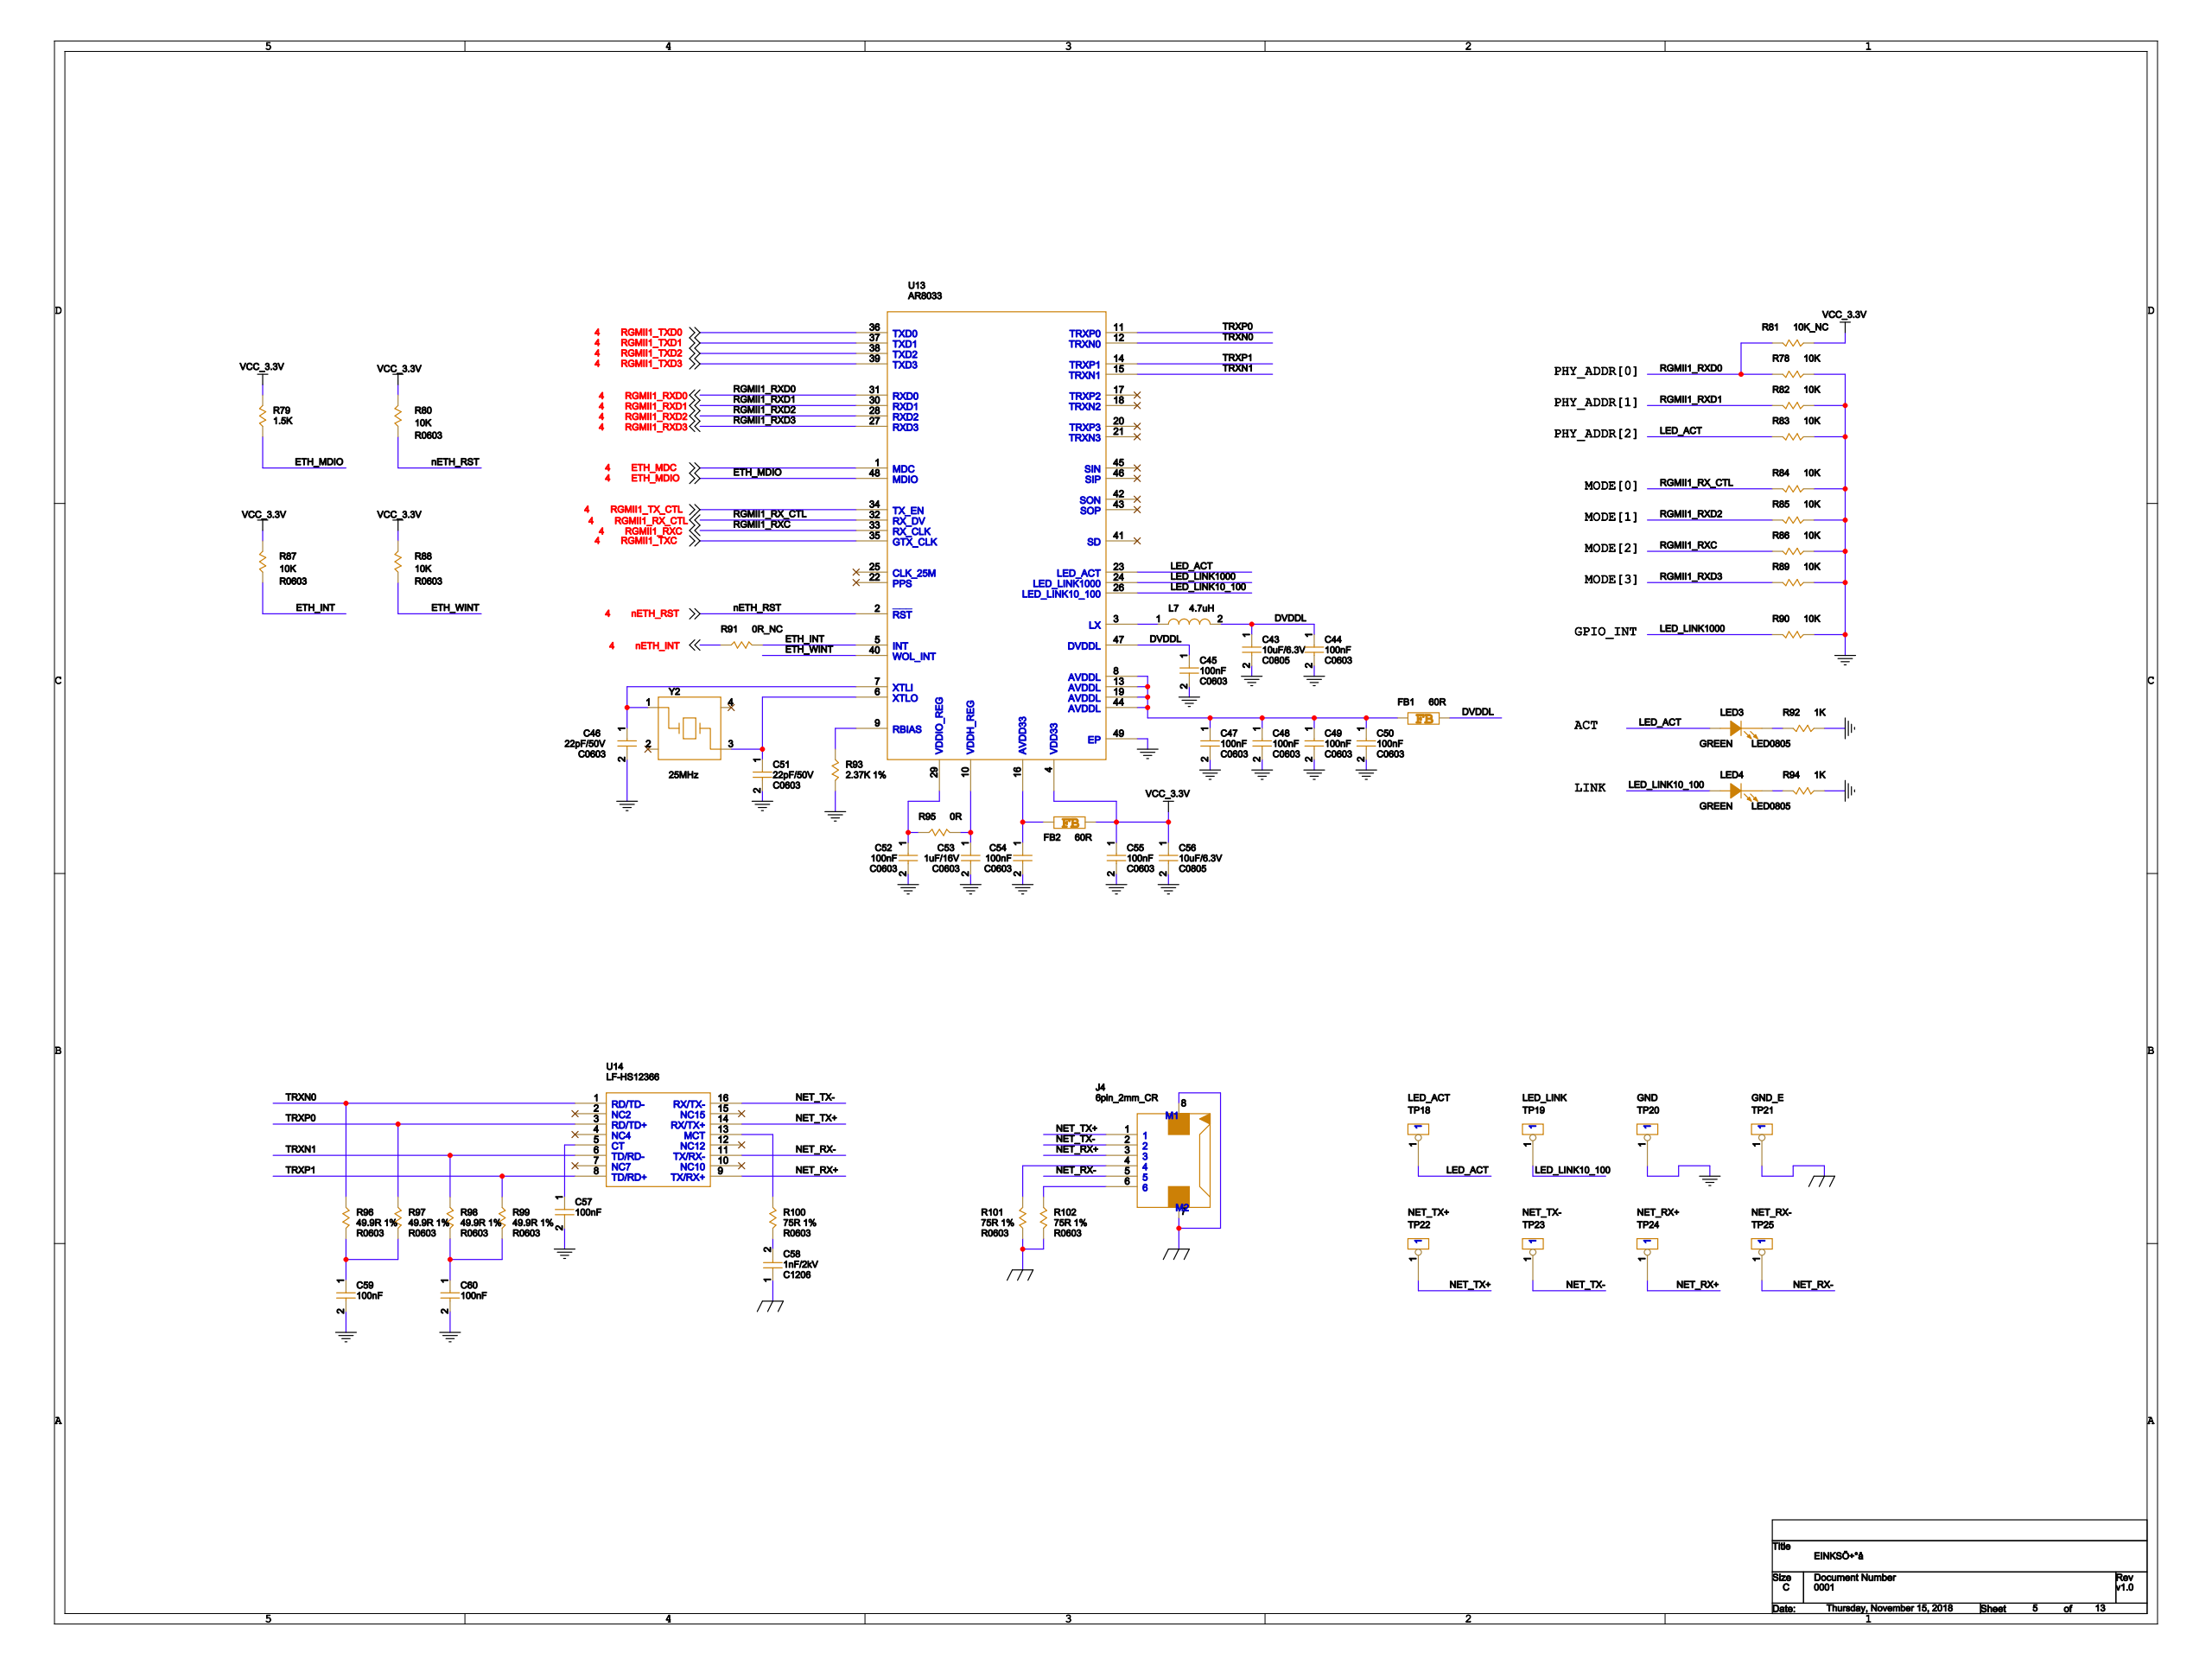Circuit board | Cadence Allegro | 609 parts | 409 nets | one sheet of the schematic
Parts on this sheet (reference | value | footprint):
C43 | 10uF/6.3V | C0805
C44 | 100nF | C0603
C45 | 100nF | C0603
C46 | 22pF/50V | C0603
C47 | 100nF | C0603
C48 | 100nF | C0603
C49 | 100nF | C0603
C50 | 100nF | C0603
C51 | 22pF/50V | C0603
C52 | 100nF | C0603
C53 | 1uF/16V | C0603
C54 | 100nF | C0603
C55 | 100nF | C0603
C56 | 10uF/6.3V | C0805
C58 | 1nF/2kV | C1206
C59 | 100nF | C0603
C60 | 100nF | C0603
FB1 | 60R | FB0603
FB2 | 60R | FB0603
J4 | 6pin_2mm_CR | PBV6_200
L7 | 4.7uH | IND_VLS3012_SM
LED3 | GREEN | LED0805
LED4 | GREEN | LED0805
R78 | 10K | R0603
R79 | 1.5K | R0603
R80 | 10K | R0603
R81 | 10K_NC | R0603
R82 | 10K | R0603
R83 | 10K | R0603
R84 | 10K | R0603
R85 | 10K | R0603
R86 | 10K | R0603
R87 | 10K | R0603
R88 | 10K | R0603
R89 | 10K | R0603
R90 | 10K | R0603
R91 | 0R_NC | R0603
R92 | 1K | R0603
R93 | 2.37K 1% | R0603
R94 | 1K | R0603
R95 | 0R | R0603
R96 | 49.9R 1% | R0603
R97 | 49.9R 1% | R0603
R98 | 49.9R 1% | R0603
R99 | 49.9R 1% | R0603
R100 | 75R 1% | R0603
R101 | 75R 1% | R0603
R102 | 75R 1% | R0603
TP18 | LED_ACT | TP_50
TP19 | LED_LINK | TP_50
TP20 | GND | TP_50
TP21 | GND_E | TP_50
TP22 | NET_TX+ | TP_50
TP23 | NET_TX- | TP_50
TP24 | NET_RX+ | TP_50
TP25 | NET_RX- | TP_50
U13 | AR8033 | QFN48P
U14 | LF-HS12366 | LF-HS12366
Y2 | 25MHz | XTAL4_SX_3225
Nets of these parts (net: part-pin ...):
GND: C43-2 C44-2 C45-2 C46-2 C47-2 C48-2 C49-2 C50-2 C51-2 C52-2 C53-2 C54-2 C55-2 C56-2 C59-2 C60-2 R78-1 R82-1 R83-1 R84-1 R85-1 R86-1 R89-1 R90-1 R92-1 R93-1 R94-1 TP20-1 U13-49
GND_E: C58-1 J4-7 J4-8 R101-2 R102-2 TP21-1
N28814691: C58-2 R100-2
VCC_3.3V: C55-1 C56-1 FB2-2 R79-1 R80-2 R81-1 R87-2 R88-2 U13-4
N28797519: C47-1 C48-1 C49-1 C50-1 FB1-1 U13-8 U13-13 U13-19 U13-44
DVDDL: C43-1 C44-1 C45-1 FB1-2 L7-2 U13-47
N28796547: C54-1 FB2-1 U13-16
NETH_INT: R91-2
NETH_RST: R80-1 U13-2
RGMII1_RXC: R86-2 U13-33
RGMII1_RXD0: R78-2 R81-2 U13-31
RGMII1_RXD1: R82-2 U13-30
RGMII1_RXD2: R85-2 U13-28
RGMII1_RXD3: R89-2 U13-27
RGMII1_RX_CTL: R84-2 U13-32
RGMII1_TXC: U13-35
RGMII1_TXD0: U13-36
RGMII1_TXD1: U13-37
RGMII1_TXD2: U13-38
RGMII1_TXD3: U13-39
ETH_MDC: U13-1
ETH_MDIO: R79-2 U13-48
RGMII1_TX_CTL: U13-34
NET_TX+: J4-1 TP22-1 U14-14
NET_TX-: J4-2 TP23-1 U14-16
NET_RX+: J4-3 TP24-1 U14-9
N28815803: J4-4 R101-1
NET_RX-: J4-5 TP25-1 U14-11
N28815808: J4-6 R102-1
N28797302: L7-1 U13-3
N28814620: R100-1 U14-13
N28788143: R93-2 U13-9
LED_ACT: LED3-2 R83-2 TP18-1 U13-23
LED_LINK10_100: LED4-2 TP19-1 U13-26
ETH_INT: R87-1 R91-1 U13-5
LED_LINK1000: R90-2 U13-24
TRXN0: R96-1 U14-1 U13-12
TRXN1: R98-1 U14-6 U13-15
TRXP0: R97-1 U14-3 U13-11
TRXP1: R99-1 U14-8 U13-14
N28795782: C53-1 R95-1 U13-10
N28795687: C52-1 R95-2 U13-29
ETH_WINT: R88-1 U13-40
N28786294: C46-1 Y2-1 U13-7
N28786971: C51-1 Y2-3 U13-6
N28814604: U14-5
N28799976: LED4-1 R94-2
N28799947: LED3-1 R92-2
N28815357: C59-1 R96-2 R97-2
N28815633: C60-1 R98-2 R99-2